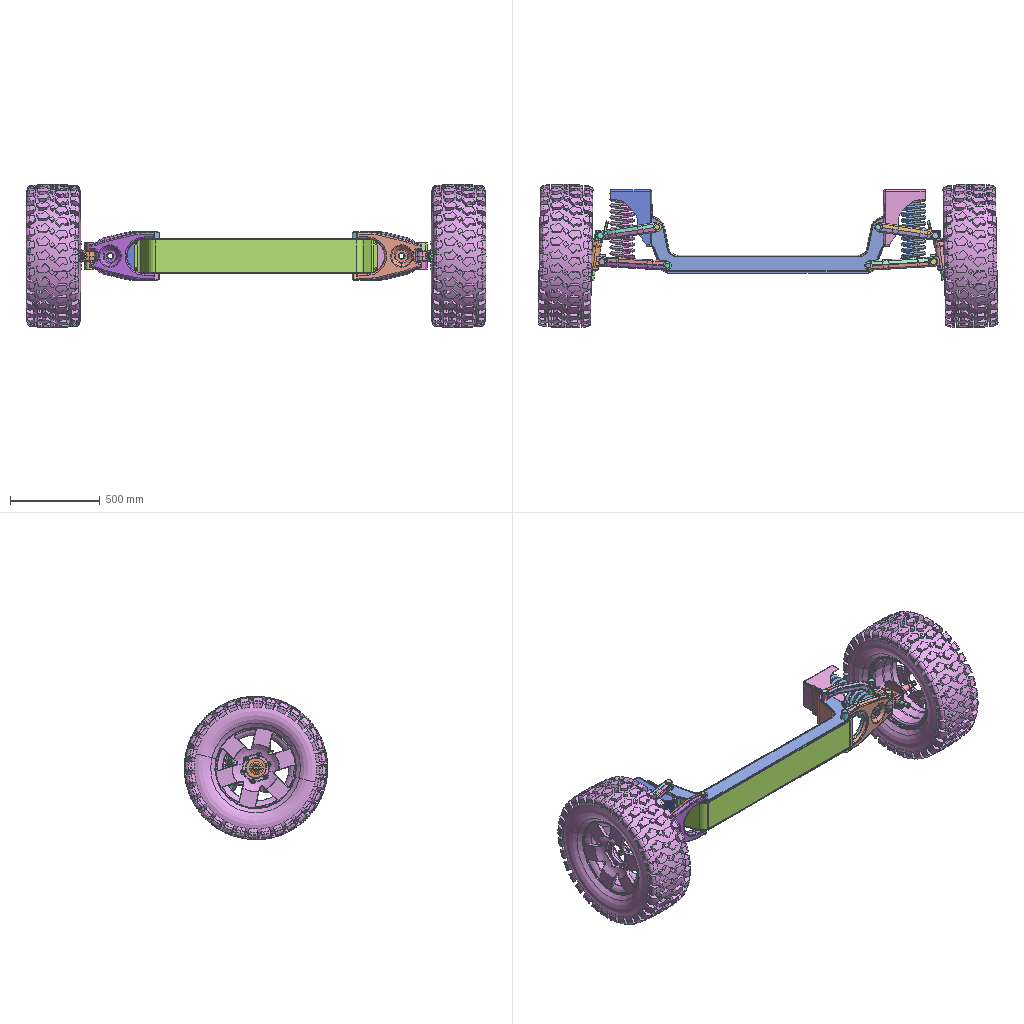Assembly | SolidWorks | 46 different items | 48 placed | box 2568 x 800 x 800 mm
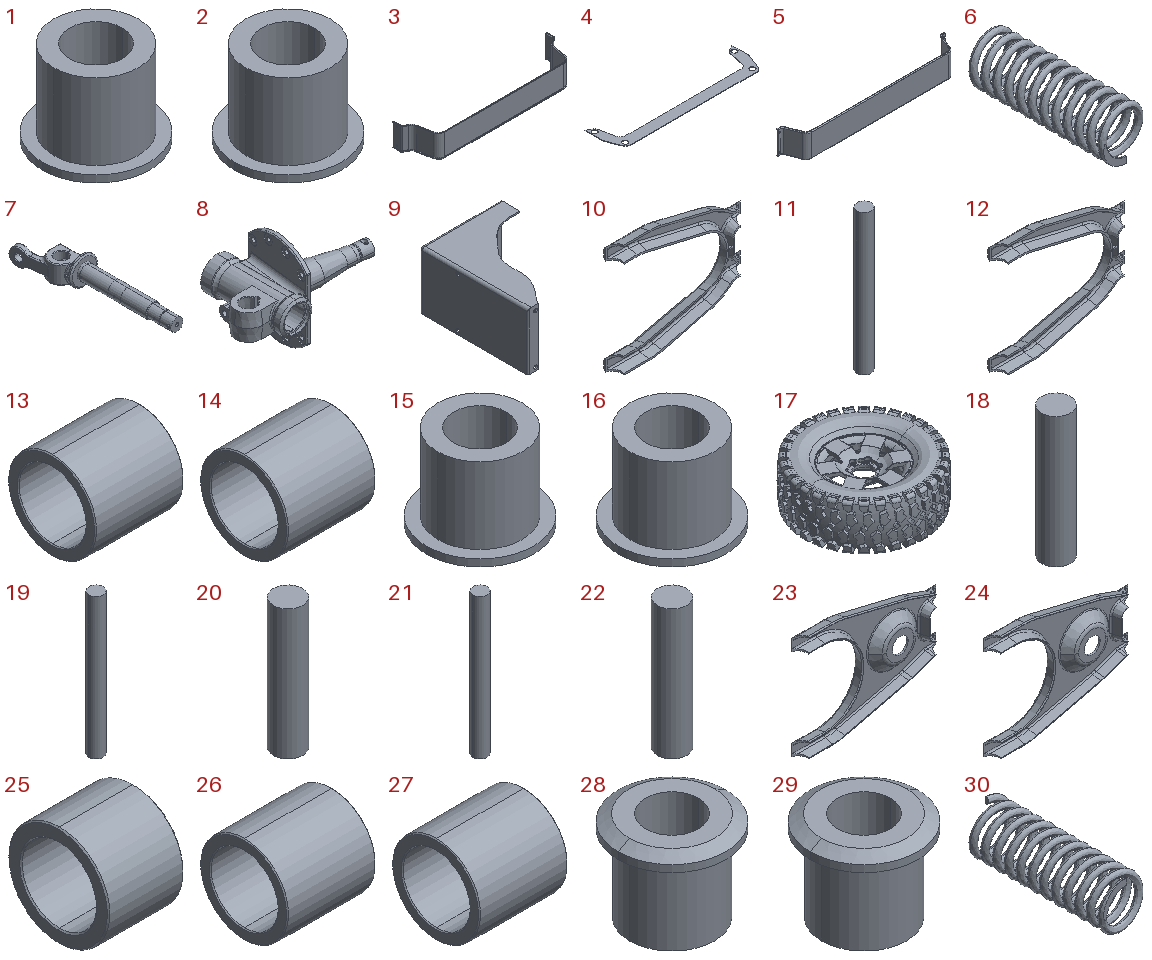Parts list (item | quantity | size | volume | features):
1 | x1 | 56.5 x 56.5 x 47 mm | 49242 mm3 | features Revolution 1
2 | x1 | 56.5 x 56.5 x 47 mm | 49242 mm3 | features Revolution 1
3 | x1 | 1308 x 294 x 192 mm | 1374323 mm3 | features ICE 13, Fillet 9, HoleWzd 2, Extrusion 1
4 | x2 | 1296 x 310.5 x 4 mm | 534691 mm3 | features Extrusion 1
5 | x1 | 1359 x 158.842 x 192 mm | 1237000 mm3 | features Fillet 8, ICE 7, Extrusion 1, HoleWzd 1
6 | x1 | 138 x 400.231 x 138 mm | 1136867 mm3 | features ICE 1, Sweep 1
7 | x1 | 83.814 x 338.849 x 64 mm | 286212 mm3 | features HoleWzd 10, 3DProfileFeature 3, Fillet 3, Chamfer 2, ICE 2, BaseBody 1, RevCut 1
8 | x1 | 266.225 x 156 x 176 mm | 686128 mm3 | features Chamfer 5, Fillet 4, HoleWzd 3, ICE 2, 3DProfileFeature 1, BaseBody 1, RevCut 1, Revolution 1, VarFillet 1
9 | x1 | 230 x 310 x 164 mm | 503816 mm3 | features Fillet 5, ICE 5, HoleWzd 2, Extrusion 1, RevCut 1, Revolution 1
10 | x1 | 321.75 x 26.25 x 270 mm | 200467 mm3 | features VarFillet 12, Fillet 2, BaseBody 1
11 | x1 | 28 x 28 x 276 mm | 169948 mm3 | features Revolution 1
12 | x1 | 321.75 x 26.25 x 270 mm | 200467 mm3 | features VarFillet 12, Fillet 2, BaseBody 1
13 | x1 | 45 x 44.5 x 44.5 mm | 29070 mm3 | features Revolution 1
14 | x1 | 45 x 44.5 x 44.5 mm | 29070 mm3 | features Revolution 1
15 | x1 | 56.5 x 56.5 x 47 mm | 49242 mm3 | features Revolution 1
16 | x1 | 56.5 x 56.5 x 47 mm | 49242 mm3 | features Revolution 1
17 | x2 | - | 94107017 mm3 | features ICE 3, Revolution 3, Fillet 2, CirPattern 1, RevCut 1
18 | x1 | 34 x 34 x 153 mm | 138912 mm3 | features MirrorStock 1
19 | x1 | 28 x 28 x 276 mm | 169948 mm3 | features MirrorStock 1
20 | x1 | 34 x 34 x 150 mm | 136188 mm3 | features MirrorStock 1
21 | x1 | 28 x 28 x 275 mm | 169332 mm3 | features MirrorStock 1
22 | x1 | 34 x 34 x 150 mm | 136188 mm3 | features Revolution 1
23 | x1 | 363.885 x 26.25 x 269.31 mm | 284905 mm3 | features MirrorStock 1
24 | x1 | 363.885 x 26.25 x 269.31 mm | 284905 mm3 | features MirrorStock 1
25 | x1 | 30 x 40 x 40 mm | 17140 mm3 | features MirrorStock 1
26 | x1 | 45 x 44.5 x 44.5 mm | 29070 mm3 | features MirrorStock 1
27 | x1 | 45 x 44.5 x 44.5 mm | 29070 mm3 | features MirrorStock 1
28 | x1 | 56.5 x 56.5 x 47 mm | 49242 mm3 | features MirrorStock 1
29 | x1 | 56.5 x 56.5 x 47 mm | 49242 mm3 | features MirrorStock 1
30 | x1 | 138 x 400.231 x 138 mm | 1136867 mm3 | features MirrorStock 1
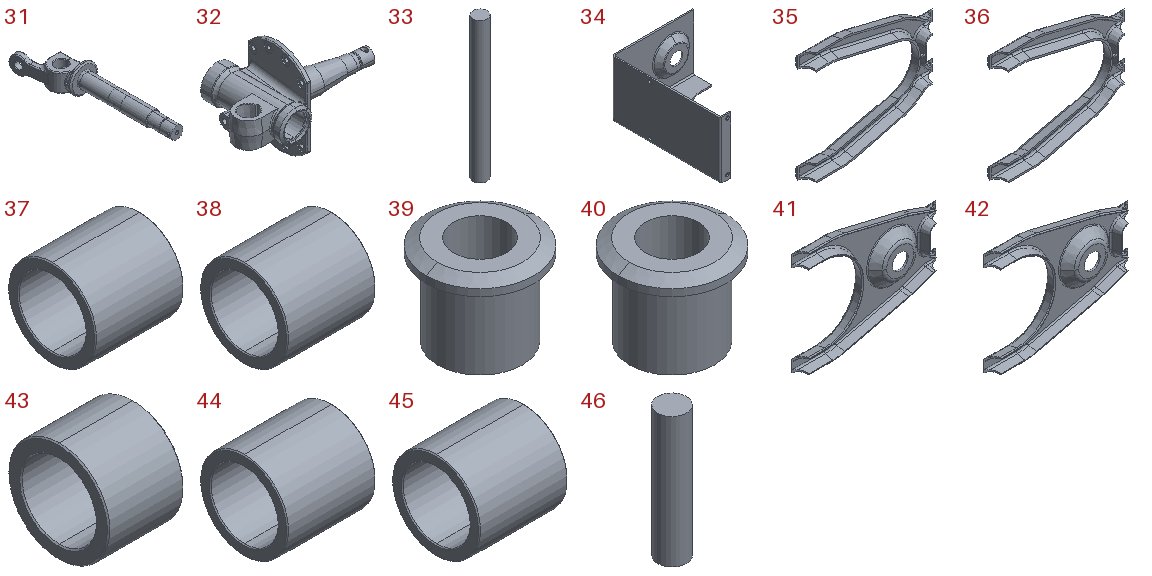31 | x1 | 83.814 x 338.849 x 64 mm | 286153 mm3 | features MirrorStock 1
32 | x1 | 266.225 x 156.001 x 176 mm | 686131 mm3 | features MirrorStock 1
33 | x1 | 28 x 28 x 275 mm | 169332 mm3 | features Revolution 1
34 | x1 | 230 x 310 x 164 mm | 503816 mm3 | features MirrorStock 1
35 | x1 | 321.75 x 26.262 x 270 mm | 200371 mm3 | features MirrorStock 1
36 | x1 | 321.75 x 26.262 x 270 mm | 200371 mm3 | features MirrorStock 1
37 | x1 | 45 x 44.5 x 44.5 mm | 29070 mm3 | features MirrorStock 1
38 | x1 | 45 x 44.5 x 44.5 mm | 29070 mm3 | features MirrorStock 1
39 | x1 | 56.5 x 56.5 x 47 mm | 49242 mm3 | features MirrorStock 1
40 | x1 | 56.5 x 56.5 x 47 mm | 49242 mm3 | features MirrorStock 1
41 | x1 | 363.885 x 26.25 x 269.31 mm | 284903 mm3 | features VarFillet 16, Fillet 3, Chamfer 2, BaseBody 1, RevCut 1, Revolution 1
42 | x1 | 363.885 x 26.25 x 269.31 mm | 284903 mm3 | features VarFillet 16, Fillet 3, Chamfer 2, BaseBody 1, RevCut 1, Revolution 1
43 | x1 | 30 x 40 x 40 mm | 17140 mm3 | features Revolution 1
44 | x1 | 45 x 44.5 x 44.5 mm | 29070 mm3 | features Revolution 1
45 | x1 | 45 x 44.5 x 44.5 mm | 29070 mm3 | features Revolution 1
46 | x1 | 34 x 34 x 153 mm | 138912 mm3 | features Revolution 1
Mates (type | each side: item.copy, entity, surface, feature):
Parallel | 3.1 face plane Cut-Extrude6 | 4.1 face plane Boss-Extrude1
Coincident | 3.1 face plane Boss-Extrude2 | 4.1 face plane Boss-Extrude1
Coincident | 3.1 face plane Boss-Extrude1 | 4.1 face plane Boss-Extrude1
Coincident | 4.1 face plane Boss-Extrude1 | 4.2 face plane Boss-Extrude1 | 2 times
Parallel | 4.1 face plane Boss-Extrude1 | 4.2 face plane Boss-Extrude1
Coincident | 3.1 face plane Boss-Extrude1 | 4.2 face plane Boss-Extrude1
Concentric | 5.1 face cylinder Ø10.0 (10) Diameter Hole1 | 9.1 face cylinder Ø10.0 (10) Diameter Hole1 | 2 times
Coincident | 5.1 face plane Boss-Extrude1 | 9.1 face plane Boss-Extrude2
Concentric | 3.1 face cylinder Ø10.0 (10) Diameter Hole2 | 9.1 face cylinder Ø10.0 (10) Diameter Hole2 | 2 times
Coincident | 3.1 face plane Cut-Extrude1 | 9.1 face plane Boss-Extrude2
Coincident | 10.1 face plane Input3 | 12.1 face plane Input3 | 3 times
Concentric | 10.1 face cylinder Input3 | 12.1 face cylinder Input3
Concentric | 4.2 face cylinder Boss-Extrude1 | 11.1 face cylinder Revolve1
Concentric | 4.1 face cylinder Boss-Extrude1 | 11.1 face cylinder Revolve1
Concentric | 11.1 face cylinder Revolve1 | 15.1 face cylinder Revolve1
Concentric | 11.1 face cylinder Revolve1 | 16.1 face cylinder Revolve1
Concentric | 10.1 face cylinder Input3 | 16.1 face cylinder Revolve1
Coincident | 4.2 face plane Boss-Extrude1 | 15.1 face plane Revolve1
Coincident | 4.1 face plane Boss-Extrude1 | 16.1 face plane Revolve1
DistanceDim | 12.1 face plane Input3 | 11.1 face plane Revolve1
DistanceDim | 11.1 face plane Revolve1 | 16.1 face plane Revolve1
Concentric | 12.1 face cylinder Input3 | 46.1 face cylinder Revolve1
Concentric | 12.1 face cylinder Input3 | 13.1 face cylinder Revolve1
Concentric | 12.1 face cylinder Input3 | 14.1 face cylinder Revolve1
DistanceDim | 12.1 face plane Input3 | 13.1 face plane Revolve1
DistanceDim | 12.1 face plane Input3 | 14.1 face plane Revolve1
DistanceDim | 46.1 face plane Revolve1 | 13.1 face plane Revolve1
Coincident | 41.1 face plane Revolve1 | 42.1 face plane Revolve1
Concentric | 41.1 face cylinder Cut-Revolve1 | 42.1 face cylinder Cut-Revolve1
Concentric | 41.1 face cylinder Input3 | 42.1 face cylinder Input3
Concentric | 41.1 face cylinder Cut-Revolve1 | 43.1 face cylinder Revolve1
DistanceDim | 43.1 face plane Revolve1 | 41.1 face plane Cut-Revolve1
Coincident | 4.2 face plane Boss-Extrude1 | 2.1 face plane Revolve1
Concentric | 4.2 face cylinder Boss-Extrude1 | 2.1 face cylinder Revolve1
Coincident | 4.1 face plane Boss-Extrude1 | 1.1 face plane Revolve1
Concentric | 4.1 face cylinder Boss-Extrude1 | 1.1 face cylinder Revolve1
Concentric | 41.1 face cylinder Input3 | 1.1 face cylinder Revolve1
Concentric | 1.1 face cylinder Revolve1 | 33.1 face cylinder Revolve1
DistanceDim | 33.1 face plane Revolve1 | 1.1 face plane Revolve1
Concentric | 42.1 face cylinder Input3 | 45.1 face cylinder Revolve1
Concentric | 42.1 face cylinder Input3 | 44.1 face cylinder Revolve1
DistanceDim | 41.1 edge | 33.1 face plane Revolve1
DistanceDim | 45.1 face plane Revolve1 | 41.1 edge
DistanceDim | 44.1 face plane Revolve1 | 41.1 edge
Concentric | 46.1 face cylinder Revolve1 | 7.1 face cylinder Input3
Concentric | 7.1 face cylinder Input3 | 8.1 face cylinder Cut-Revolve1
Coincident | 7.1 face plane Input3 | 8.1 face plane Input3
DistanceDim | 7.1 face plane Input3 | 13.1 face plane Revolve1
Concentric | 45.1 face cylinder Revolve1 | 8.1 face cone Input3
Concentric | 9.1 face cylinder Cut-Revolve1 | 6.1 select_type:24
Concentric | 45.1 face cylinder Revolve1 | 22.1 face cylinder Revolve1
Coincident | 44.1 face plane Revolve1 | 22.1 face plane Revolve1
Concentric | 8.1 face cylinder Revolve1 | 17.1 face cylinder Revolve1
DistanceDim | 8.1 face plane Revolve1 | 17.1 face plane Revolve1